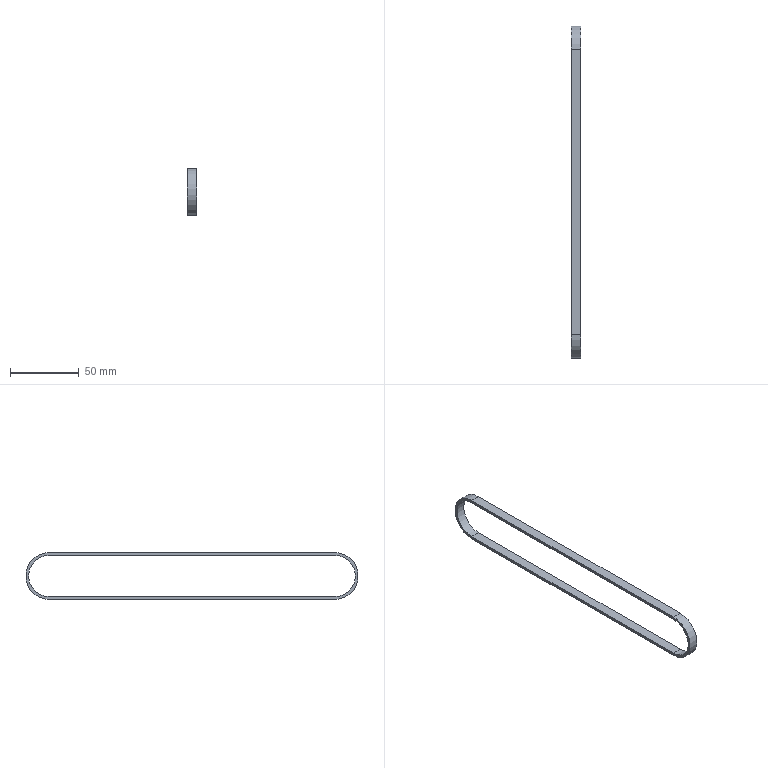Part | NX | features DATUM_CSYS 2, EXTRUDE 1, SKETCH 1 | 1 solid | 10 faces | box 7 x 241.055 x 34 mm | volume 7205 mm3 | plane 6 | cylinder 4 | commonest cylinder face diameters 30 x2 34 x2
STEP:
#1=CARTESIAN_POINT('',(7.,103.528,-17.));
#2=VERTEX_POINT('',#1);
#3=CARTESIAN_POINT('',(7.,103.528,17.));
#4=VERTEX_POINT('',#3);
#5=CARTESIAN_POINT('',(7.,103.528,0.));
#6=DIRECTION('',(1.,0.,0.));
#7=DIRECTION('',(0.,0.,-1.));
#8=AXIS2_PLACEMENT_3D('',#5,#6,#7);
#9=CIRCLE('',#8,17.);
#10=EDGE_CURVE('',#2,#4,#9,.T.);
#11=ORIENTED_EDGE('',*,*,#10,.T.);
#12=CARTESIAN_POINT('',(7.,-103.528,17.));
#13=VERTEX_POINT('',#12);
#14=CARTESIAN_POINT('',(7.,103.528,17.));
#15=DIRECTION('',(0.,1.,0.));
#16=VECTOR('',#15,1000.);
#17=LINE('',#14,#16);
#18=EDGE_CURVE('',#4,#13,#17,.F.);
#19=ORIENTED_EDGE('',*,*,#18,.T.);
#20=CARTESIAN_POINT('',(7.,-103.528,-17.));
#21=VERTEX_POINT('',#20);
#22=CARTESIAN_POINT('',(7.,-103.528,0.));
#23=DIRECTION('',(1.,0.,0.));
#24=DIRECTION('',(0.,0.,-1.));
#25=AXIS2_PLACEMENT_3D('',#22,#23,#24);
#26=CIRCLE('',#25,17.);
#27=EDGE_CURVE('',#13,#21,#26,.T.);
#28=ORIENTED_EDGE('',*,*,#27,.T.);
#29=CARTESIAN_POINT('',(7.,-103.528,-17.));
#30=DIRECTION('',(0.,1.,0.));
#31=VECTOR('',#30,1000.);
#32=LINE('',#29,#31);
#33=EDGE_CURVE('',#21,#2,#32,.T.);
#34=ORIENTED_EDGE('',*,*,#33,.T.);
#35=EDGE_LOOP('',(#11,#19,#28,#34));
#36=FACE_BOUND('',#35,.T.);
#37=CARTESIAN_POINT('',(7.,103.528,-15.));
#38=VERTEX_POINT('',#37);
#39=CARTESIAN_POINT('',(7.,103.528,15.));
#40=VERTEX_POINT('',#39);
#41=CARTESIAN_POINT('',(7.,103.528,0.));
#42=DIRECTION('',(1.,0.,0.));
#43=DIRECTION('',(0.,1.,0.));
#44=AXIS2_PLACEMENT_3D('',#41,#42,#43);
#45=CIRCLE('',#44,15.);
#46=EDGE_CURVE('',#38,#40,#45,.T.);
#47=ORIENTED_EDGE('',*,*,#46,.F.);
#48=CARTESIAN_POINT('',(7.,-103.528,-15.));
#49=VERTEX_POINT('',#48);
#50=CARTESIAN_POINT('',(7.,-103.528,-15.));
#51=DIRECTION('',(0.,1.,0.));
#52=VECTOR('',#51,1000.);
#53=LINE('',#50,#52);
#54=EDGE_CURVE('',#49,#38,#53,.T.);
#55=ORIENTED_EDGE('',*,*,#54,.F.);
#56=CARTESIAN_POINT('',(7.,-103.528,15.));
#57=VERTEX_POINT('',#56);
#58=CARTESIAN_POINT('',(7.,-103.528,0.));
#59=DIRECTION('',(1.,0.,0.));
#60=DIRECTION('',(0.,1.,0.));
#61=AXIS2_PLACEMENT_3D('',#58,#59,#60);
#62=CIRCLE('',#61,15.);
#63=EDGE_CURVE('',#57,#49,#62,.T.);
#64=ORIENTED_EDGE('',*,*,#63,.F.);
#65=CARTESIAN_POINT('',(7.,103.528,15.));
#66=DIRECTION('',(0.,-1.,0.));
#67=VECTOR('',#66,1000.);
#68=LINE('',#65,#67);
#69=EDGE_CURVE('',#40,#57,#68,.T.);
#70=ORIENTED_EDGE('',*,*,#69,.F.);
#71=EDGE_LOOP('',(#47,#55,#64,#70));
#72=FACE_BOUND('',#71,.T.);
#73=CARTESIAN_POINT('',(7.,103.528,0.));
#74=DIRECTION('',(-1.,0.,0.));
#75=DIRECTION('',(0.,0.,1.));
#76=AXIS2_PLACEMENT_3D('',#73,#74,#75);
#77=PLANE('',#76);
#78=ADVANCED_FACE('',(#36,#72),#77,.F.);
#79=CARTESIAN_POINT('',(0.,-103.528,17.));
#80=VERTEX_POINT('',#79);
#81=CARTESIAN_POINT('',(0.,-103.528,-17.));
#82=VERTEX_POINT('',#81);
#83=CARTESIAN_POINT('',(0.,-103.528,0.));
#84=DIRECTION('',(1.,0.,0.));
#85=DIRECTION('',(0.,0.,-1.));
#86=AXIS2_PLACEMENT_3D('',#83,#84,#85);
#87=CIRCLE('',#86,17.);
#88=EDGE_CURVE('',#80,#82,#87,.T.);
#89=ORIENTED_EDGE('',*,*,#88,.F.);
#90=CARTESIAN_POINT('',(0.,103.528,17.));
#91=VERTEX_POINT('',#90);
#92=CARTESIAN_POINT('',(0.,103.528,17.));
#93=DIRECTION('',(0.,1.,0.));
#94=VECTOR('',#93,1000.);
#95=LINE('',#92,#94);
#96=EDGE_CURVE('',#91,#80,#95,.F.);
#97=ORIENTED_EDGE('',*,*,#96,.F.);
#98=CARTESIAN_POINT('',(0.,103.528,-17.));
#99=VERTEX_POINT('',#98);
#100=CARTESIAN_POINT('',(0.,103.528,0.));
#101=DIRECTION('',(1.,0.,0.));
#102=DIRECTION('',(0.,0.,-1.));
#103=AXIS2_PLACEMENT_3D('',#100,#101,#102);
#104=CIRCLE('',#103,17.);
#105=EDGE_CURVE('',#99,#91,#104,.T.);
#106=ORIENTED_EDGE('',*,*,#105,.F.);
#107=CARTESIAN_POINT('',(0.,-103.528,-17.));
#108=DIRECTION('',(0.,1.,0.));
#109=VECTOR('',#108,1000.);
#110=LINE('',#107,#109);
#111=EDGE_CURVE('',#82,#99,#110,.T.);
#112=ORIENTED_EDGE('',*,*,#111,.F.);
#113=EDGE_LOOP('',(#89,#97,#106,#112));
#114=FACE_BOUND('',#113,.T.);
#115=CARTESIAN_POINT('',(0.,-103.528,15.));
#116=VERTEX_POINT('',#115);
#117=CARTESIAN_POINT('',(0.,-103.528,-15.));
#118=VERTEX_POINT('',#117);
#119=CARTESIAN_POINT('',(0.,-103.528,0.));
#120=DIRECTION('',(1.,0.,0.));
#121=DIRECTION('',(0.,1.,0.));
#122=AXIS2_PLACEMENT_3D('',#119,#120,#121);
#123=CIRCLE('',#122,15.);
#124=EDGE_CURVE('',#116,#118,#123,.T.);
#125=ORIENTED_EDGE('',*,*,#124,.T.);
#126=CARTESIAN_POINT('',(0.,103.528,-15.));
#127=VERTEX_POINT('',#126);
#128=CARTESIAN_POINT('',(0.,-103.528,-15.));
#129=DIRECTION('',(0.,1.,0.));
#130=VECTOR('',#129,1000.);
#131=LINE('',#128,#130);
#132=EDGE_CURVE('',#118,#127,#131,.T.);
#133=ORIENTED_EDGE('',*,*,#132,.T.);
#134=CARTESIAN_POINT('',(0.,103.528,15.));
#135=VERTEX_POINT('',#134);
#136=CARTESIAN_POINT('',(0.,103.528,0.));
#137=DIRECTION('',(1.,0.,0.));
#138=DIRECTION('',(0.,1.,0.));
#139=AXIS2_PLACEMENT_3D('',#136,#137,#138);
#140=CIRCLE('',#139,15.);
#141=EDGE_CURVE('',#127,#135,#140,.T.);
#142=ORIENTED_EDGE('',*,*,#141,.T.);
#143=CARTESIAN_POINT('',(0.,103.528,15.));
#144=DIRECTION('',(0.,-1.,0.));
#145=VECTOR('',#144,1000.);
#146=LINE('',#143,#145);
#147=EDGE_CURVE('',#135,#116,#146,.T.);
#148=ORIENTED_EDGE('',*,*,#147,.T.);
#149=EDGE_LOOP('',(#125,#133,#142,#148));
#150=FACE_BOUND('',#149,.T.);
#151=CARTESIAN_POINT('',(0.,-103.528,0.));
#152=DIRECTION('',(-1.,0.,0.));
#153=DIRECTION('',(0.,0.,1.));
#154=AXIS2_PLACEMENT_3D('',#151,#152,#153);
#155=PLANE('',#154);
#156=ADVANCED_FACE('',(#114,#150),#155,.T.);
#157=ORIENTED_EDGE('',*,*,#18,.F.);
#158=CARTESIAN_POINT('',(0.,103.528,17.));
#159=DIRECTION('',(1.,0.,0.));
#160=VECTOR('',#159,1000.);
#161=LINE('',#158,#160);
#162=EDGE_CURVE('',#91,#4,#161,.T.);
#163=ORIENTED_EDGE('',*,*,#162,.F.);
#164=ORIENTED_EDGE('',*,*,#96,.T.);
#165=CARTESIAN_POINT('',(0.,-103.528,17.));
#166=DIRECTION('',(1.,0.,0.));
#167=VECTOR('',#166,1000.);
#168=LINE('',#165,#167);
#169=EDGE_CURVE('',#80,#13,#168,.T.);
#170=ORIENTED_EDGE('',*,*,#169,.T.);
#171=EDGE_LOOP('',(#157,#163,#164,#170));
#172=FACE_BOUND('',#171,.T.);
#173=CARTESIAN_POINT('',(0.,103.528,17.));
#174=DIRECTION('',(0.,0.,1.));
#175=DIRECTION('',(1.,0.,0.));
#176=AXIS2_PLACEMENT_3D('',#173,#174,#175);
#177=PLANE('',#176);
#178=ADVANCED_FACE('',(#172),#177,.T.);
#179=ORIENTED_EDGE('',*,*,#27,.F.);
#180=ORIENTED_EDGE('',*,*,#169,.F.);
#181=ORIENTED_EDGE('',*,*,#88,.T.);
#182=CARTESIAN_POINT('',(0.,-103.528,-17.));
#183=DIRECTION('',(1.,0.,0.));
#184=VECTOR('',#183,1000.);
#185=LINE('',#182,#184);
#186=EDGE_CURVE('',#82,#21,#185,.T.);
#187=ORIENTED_EDGE('',*,*,#186,.T.);
#188=EDGE_LOOP('',(#179,#180,#181,#187));
#189=FACE_BOUND('',#188,.T.);
#190=CARTESIAN_POINT('',(0.,-103.528,0.));
#191=DIRECTION('',(1.,0.,0.));
#192=DIRECTION('',(0.,0.,-1.));
#193=AXIS2_PLACEMENT_3D('',#190,#191,#192);
#194=CYLINDRICAL_SURFACE('',#193,17.);
#195=ADVANCED_FACE('',(#189),#194,.T.);
#196=ORIENTED_EDGE('',*,*,#33,.F.);
#197=ORIENTED_EDGE('',*,*,#186,.F.);
#198=ORIENTED_EDGE('',*,*,#111,.T.);
#199=CARTESIAN_POINT('',(0.,103.528,-17.));
#200=DIRECTION('',(-1.,0.,0.));
#201=VECTOR('',#200,1000.);
#202=LINE('',#199,#201);
#203=EDGE_CURVE('',#99,#2,#202,.F.);
#204=ORIENTED_EDGE('',*,*,#203,.T.);
#205=EDGE_LOOP('',(#196,#197,#198,#204));
#206=FACE_BOUND('',#205,.T.);
#207=CARTESIAN_POINT('',(0.,-103.528,-17.));
#208=DIRECTION('',(0.,0.,-1.));
#209=DIRECTION('',(-1.,0.,0.));
#210=AXIS2_PLACEMENT_3D('',#207,#208,#209);
#211=PLANE('',#210);
#212=ADVANCED_FACE('',(#206),#211,.T.);
#213=ORIENTED_EDGE('',*,*,#10,.F.);
#214=ORIENTED_EDGE('',*,*,#203,.F.);
#215=ORIENTED_EDGE('',*,*,#105,.T.);
#216=ORIENTED_EDGE('',*,*,#162,.T.);
#217=EDGE_LOOP('',(#213,#214,#215,#216));
#218=FACE_BOUND('',#217,.T.);
#219=CARTESIAN_POINT('',(0.,103.528,0.));
#220=DIRECTION('',(1.,0.,0.));
#221=DIRECTION('',(0.,0.,-1.));
#222=AXIS2_PLACEMENT_3D('',#219,#220,#221);
#223=CYLINDRICAL_SURFACE('',#222,17.);
#224=ADVANCED_FACE('',(#218),#223,.T.);
#225=ORIENTED_EDGE('',*,*,#69,.T.);
#226=CARTESIAN_POINT('',(0.,-103.528,15.));
#227=DIRECTION('',(1.,0.,0.));
#228=VECTOR('',#227,1000.);
#229=LINE('',#226,#228);
#230=EDGE_CURVE('',#116,#57,#229,.T.);
#231=ORIENTED_EDGE('',*,*,#230,.F.);
#232=ORIENTED_EDGE('',*,*,#147,.F.);
#233=CARTESIAN_POINT('',(0.,103.528,15.));
#234=DIRECTION('',(1.,0.,0.));
#235=VECTOR('',#234,1000.);
#236=LINE('',#233,#235);
#237=EDGE_CURVE('',#135,#40,#236,.T.);
#238=ORIENTED_EDGE('',*,*,#237,.T.);
#239=EDGE_LOOP('',(#225,#231,#232,#238));
#240=FACE_BOUND('',#239,.T.);
#241=CARTESIAN_POINT('',(0.,103.528,15.));
#242=DIRECTION('',(0.,0.,1.));
#243=DIRECTION('',(1.,0.,0.));
#244=AXIS2_PLACEMENT_3D('',#241,#242,#243);
#245=PLANE('',#244);
#246=ADVANCED_FACE('',(#240),#245,.F.);
#247=ORIENTED_EDGE('',*,*,#63,.T.);
#248=CARTESIAN_POINT('',(0.,-103.528,-15.));
#249=DIRECTION('',(1.,0.,0.));
#250=VECTOR('',#249,1000.);
#251=LINE('',#248,#250);
#252=EDGE_CURVE('',#118,#49,#251,.T.);
#253=ORIENTED_EDGE('',*,*,#252,.F.);
#254=ORIENTED_EDGE('',*,*,#124,.F.);
#255=ORIENTED_EDGE('',*,*,#230,.T.);
#256=EDGE_LOOP('',(#247,#253,#254,#255));
#257=FACE_BOUND('',#256,.T.);
#258=CARTESIAN_POINT('',(0.,-103.528,0.));
#259=DIRECTION('',(1.,0.,0.));
#260=DIRECTION('',(0.,0.,-1.));
#261=AXIS2_PLACEMENT_3D('',#258,#259,#260);
#262=CYLINDRICAL_SURFACE('',#261,15.);
#263=ADVANCED_FACE('',(#257),#262,.F.);
#264=ORIENTED_EDGE('',*,*,#54,.T.);
#265=CARTESIAN_POINT('',(0.,103.528,-15.));
#266=DIRECTION('',(1.,0.,0.));
#267=VECTOR('',#266,1000.);
#268=LINE('',#265,#267);
#269=EDGE_CURVE('',#127,#38,#268,.T.);
#270=ORIENTED_EDGE('',*,*,#269,.F.);
#271=ORIENTED_EDGE('',*,*,#132,.F.);
#272=ORIENTED_EDGE('',*,*,#252,.T.);
#273=EDGE_LOOP('',(#264,#270,#271,#272));
#274=FACE_BOUND('',#273,.T.);
#275=CARTESIAN_POINT('',(0.,-103.528,-15.));
#276=DIRECTION('',(0.,0.,-1.));
#277=DIRECTION('',(-1.,0.,0.));
#278=AXIS2_PLACEMENT_3D('',#275,#276,#277);
#279=PLANE('',#278);
#280=ADVANCED_FACE('',(#274),#279,.F.);
#281=ORIENTED_EDGE('',*,*,#46,.T.);
#282=ORIENTED_EDGE('',*,*,#237,.F.);
#283=ORIENTED_EDGE('',*,*,#141,.F.);
#284=ORIENTED_EDGE('',*,*,#269,.T.);
#285=EDGE_LOOP('',(#281,#282,#283,#284));
#286=FACE_BOUND('',#285,.T.);
#287=CARTESIAN_POINT('',(0.,103.528,0.));
#288=DIRECTION('',(1.,0.,0.));
#289=DIRECTION('',(0.,0.,-1.));
#290=AXIS2_PLACEMENT_3D('',#287,#288,#289);
#291=CYLINDRICAL_SURFACE('',#290,15.);
#292=ADVANCED_FACE('',(#286),#291,.F.);
#293=CLOSED_SHELL('',(#78,#156,#178,#195,#212,#224,#246,#263,#280,#292));
#294=MANIFOLD_SOLID_BREP('',#293);
#295=(LENGTH_UNIT()NAMED_UNIT(*)SI_UNIT(.MILLI.,.METRE.));
#296=UNCERTAINTY_MEASURE_WITH_UNIT(LENGTH_MEASURE(0.00001),#295,'','');
#297=(NAMED_UNIT(*)PLANE_ANGLE_UNIT()SI_UNIT($,.RADIAN.));
#298=(NAMED_UNIT(*)SI_UNIT($,.STERADIAN.)SOLID_ANGLE_UNIT());
#299=(GEOMETRIC_REPRESENTATION_CONTEXT(3)GLOBAL_UNCERTAINTY_ASSIGNED_CONTEXT((#296))GLOBAL_UNIT_ASSIGNED_CONTEXT((#295,#297,#298))REPRESENTATION_CONTEXT('',''));
#300=ADVANCED_BREP_SHAPE_REPRESENTATION('',(#294),#299);